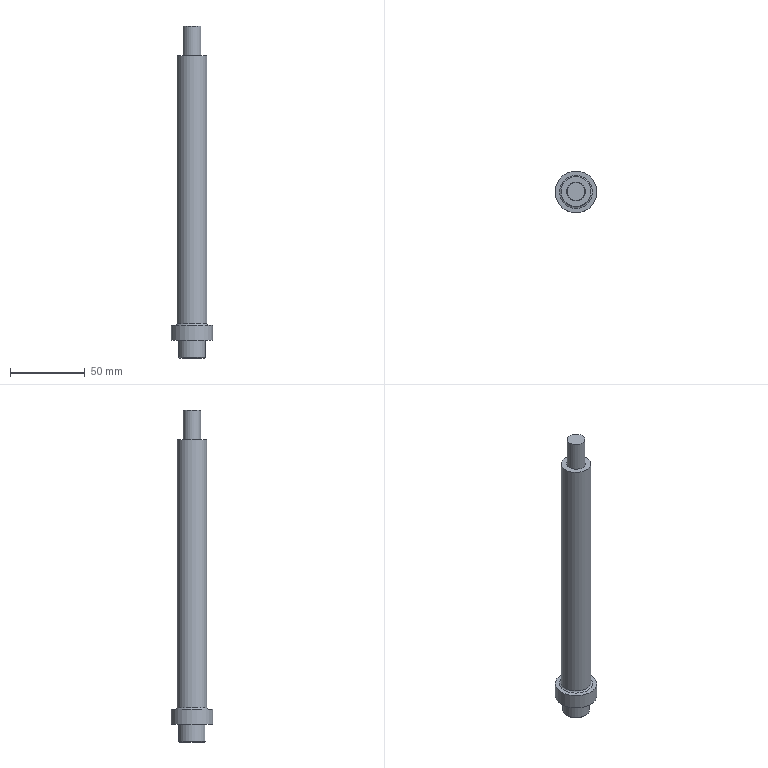Part | STEP file | 1_id3750_x_t | 1 solid | 29 faces | box 28 x 28 x 222 mm | volume 65272 mm3 | plane 18 | cylinder 6 | cone 4 | torus 1 | commonest cylinder face diameters 12.6 x2 12 x1 18 x1 20 x1 28 x1
STEP:
#1=CARTESIAN_POINT('',(2798.,0.00007613,-220.));
#2=VERTEX_POINT('',#1);
#3=CARTESIAN_POINT('',(2787.,0.00007613,-220.));
#4=DIRECTION('',(0.,0.,1.));
#5=DIRECTION('',(1.,0.,0.));
#6=AXIS2_PLACEMENT_3D('',#3,#4,#5);
#7=CIRCLE('',#6,11.);
#8=EDGE_CURVE('',#2,#2,#7,.T.);
#9=ORIENTED_EDGE('',*,*,#8,.T.);
#10=EDGE_LOOP('',(#9));
#11=FACE_BOUND('',#10,.T.);
#12=CARTESIAN_POINT('',(2797.,0.00007613,-219.));
#13=VERTEX_POINT('',#12);
#14=CARTESIAN_POINT('',(2787.,0.00007613,-219.));
#15=DIRECTION('',(0.,0.,-1.));
#16=DIRECTION('',(1.,0.,0.));
#17=AXIS2_PLACEMENT_3D('',#14,#15,#16);
#18=CIRCLE('',#17,10.);
#19=EDGE_CURVE('',#13,#13,#18,.T.);
#20=ORIENTED_EDGE('',*,*,#19,.T.);
#21=EDGE_LOOP('',(#20));
#22=FACE_BOUND('',#21,.T.);
#23=CARTESIAN_POINT('',(2787.,0.00007613,-219.));
#24=DIRECTION('',(0.,0.,-1.));
#25=DIRECTION('',(-1.,0.,0.));
#26=AXIS2_PLACEMENT_3D('',#23,#24,#25);
#27=TOROIDAL_SURFACE('',#26,11.,1.);
#28=ADVANCED_FACE('',(#11,#22),#27,.F.);
#29=CARTESIAN_POINT('',(2773.,0.00007613,-230.));
#30=VERTEX_POINT('',#29);
#31=CARTESIAN_POINT('',(2787.,0.00007613,-230.));
#32=DIRECTION('',(0.,0.,-1.));
#33=DIRECTION('',(-1.,0.,0.));
#34=AXIS2_PLACEMENT_3D('',#31,#32,#33);
#35=CIRCLE('',#34,14.);
#36=EDGE_CURVE('',#30,#30,#35,.T.);
#37=ORIENTED_EDGE('',*,*,#36,.F.);
#38=EDGE_LOOP('',(#37));
#39=FACE_BOUND('',#38,.T.);
#40=CARTESIAN_POINT('',(2773.,0.00007613,-220.));
#41=VERTEX_POINT('',#40);
#42=CARTESIAN_POINT('',(2787.,0.00007613,-220.));
#43=DIRECTION('',(0.,0.,1.));
#44=DIRECTION('',(-1.,0.,0.));
#45=AXIS2_PLACEMENT_3D('',#42,#43,#44);
#46=CIRCLE('',#45,14.);
#47=EDGE_CURVE('',#41,#41,#46,.T.);
#48=ORIENTED_EDGE('',*,*,#47,.F.);
#49=EDGE_LOOP('',(#48));
#50=FACE_BOUND('',#49,.T.);
#51=CARTESIAN_POINT('',(2787.,0.00007613,-225.));
#52=DIRECTION('',(0.,0.,1.));
#53=DIRECTION('',(1.,0.,0.));
#54=AXIS2_PLACEMENT_3D('',#51,#52,#53);
#55=CYLINDRICAL_SURFACE('',#54,14.);
#56=ADVANCED_FACE('',(#39,#50),#55,.T.);
#57=CARTESIAN_POINT('',(2780.7,0.00007613,-40.));
#58=VERTEX_POINT('',#57);
#59=CARTESIAN_POINT('',(2780.7,0.00007613,-230.));
#60=VERTEX_POINT('',#59);
#61=CARTESIAN_POINT('',(2780.7,0.00007613,-95.));
#62=DIRECTION('',(0.,0.,-1.));
#63=VECTOR('',#62,1.);
#64=LINE('',#61,#63);
#65=EDGE_CURVE('',#58,#60,#64,.T.);
#66=ORIENTED_EDGE('',*,*,#65,.F.);
#67=CARTESIAN_POINT('',(2793.3,0.00007613,-40.));
#68=VERTEX_POINT('',#67);
#69=CARTESIAN_POINT('',(2787.,0.00007613,-40.));
#70=DIRECTION('',(0.,0.,-1.));
#71=DIRECTION('',(-1.,0.,0.));
#72=AXIS2_PLACEMENT_3D('',#69,#70,#71);
#73=CIRCLE('',#72,6.3);
#74=EDGE_CURVE('',#68,#58,#73,.T.);
#75=ORIENTED_EDGE('',*,*,#74,.F.);
#76=CARTESIAN_POINT('',(2793.3,0.00007613,-230.));
#77=VERTEX_POINT('',#76);
#78=CARTESIAN_POINT('',(2793.3,0.00007613,-95.));
#79=DIRECTION('',(0.,0.,1.));
#80=VECTOR('',#79,1.);
#81=LINE('',#78,#80);
#82=EDGE_CURVE('',#77,#68,#81,.T.);
#83=ORIENTED_EDGE('',*,*,#82,.F.);
#84=CARTESIAN_POINT('',(2787.,0.00007613,-230.));
#85=DIRECTION('',(0.,0.,1.));
#86=DIRECTION('',(-1.,0.,0.));
#87=AXIS2_PLACEMENT_3D('',#84,#85,#86);
#88=CIRCLE('',#87,6.3);
#89=EDGE_CURVE('',#60,#77,#88,.T.);
#90=ORIENTED_EDGE('',*,*,#89,.F.);
#91=EDGE_LOOP('',(#66,#75,#83,#90));
#92=FACE_OUTER_BOUND('',#91,.T.);
#93=CARTESIAN_POINT('',(2787.,0.00007613,-95.));
#94=DIRECTION('',(0.,0.,1.));
#95=DIRECTION('',(1.,0.,0.));
#96=AXIS2_PLACEMENT_3D('',#93,#94,#95);
#97=CYLINDRICAL_SURFACE('',#96,6.3);
#98=ADVANCED_FACE('',(#92),#97,.F.);
#99=ORIENTED_EDGE('',*,*,#19,.F.);
#100=EDGE_LOOP('',(#99));
#101=FACE_BOUND('',#100,.T.);
#102=CARTESIAN_POINT('',(2777.,0.00007613,-40.));
#103=VERTEX_POINT('',#102);
#104=CARTESIAN_POINT('',(2787.,0.00007613,-40.));
#105=DIRECTION('',(0.,0.,1.));
#106=DIRECTION('',(-1.,0.,0.));
#107=AXIS2_PLACEMENT_3D('',#104,#105,#106);
#108=CIRCLE('',#107,10.);
#109=EDGE_CURVE('',#103,#103,#108,.T.);
#110=ORIENTED_EDGE('',*,*,#109,.F.);
#111=EDGE_LOOP('',(#110));
#112=FACE_BOUND('',#111,.T.);
#113=CARTESIAN_POINT('',(2787.,0.00007613,-90.));
#114=DIRECTION('',(0.,0.,1.));
#115=DIRECTION('',(1.,0.,0.));
#116=AXIS2_PLACEMENT_3D('',#113,#114,#115);
#117=CYLINDRICAL_SURFACE('',#116,10.);
#118=ADVANCED_FACE('',(#101,#112),#117,.T.);
#119=CARTESIAN_POINT('',(2781.,0.00007613,-230.));
#120=VERTEX_POINT('',#119);
#121=CARTESIAN_POINT('',(2787.,0.00007613,-230.));
#122=DIRECTION('',(0.,0.,-1.));
#123=DIRECTION('',(-1.,0.,0.));
#124=AXIS2_PLACEMENT_3D('',#121,#122,#123);
#125=CIRCLE('',#124,6.);
#126=EDGE_CURVE('',#120,#120,#125,.T.);
#127=ORIENTED_EDGE('',*,*,#126,.F.);
#128=EDGE_LOOP('',(#127));
#129=FACE_BOUND('',#128,.T.);
#130=CARTESIAN_POINT('',(2781.,0.00007613,-20.));
#131=VERTEX_POINT('',#130);
#132=CARTESIAN_POINT('',(2787.,0.00007613,-20.));
#133=DIRECTION('',(0.,0.,1.));
#134=DIRECTION('',(-1.,0.,0.));
#135=AXIS2_PLACEMENT_3D('',#132,#133,#134);
#136=CIRCLE('',#135,6.);
#137=EDGE_CURVE('',#131,#131,#136,.T.);
#138=ORIENTED_EDGE('',*,*,#137,.F.);
#139=EDGE_LOOP('',(#138));
#140=FACE_BOUND('',#139,.T.);
#141=CARTESIAN_POINT('',(2787.,0.00007613,-85.));
#142=DIRECTION('',(0.,0.,1.));
#143=DIRECTION('',(1.,0.,0.));
#144=AXIS2_PLACEMENT_3D('',#141,#142,#143);
#145=CYLINDRICAL_SURFACE('',#144,6.);
#146=ADVANCED_FACE('',(#129,#140),#145,.T.);
#147=CARTESIAN_POINT('',(2792.774,0.00007613,-236.));
#148=VERTEX_POINT('',#147);
#149=CARTESIAN_POINT('',(2787.,0.00007613,-235.));
#150=VERTEX_POINT('',#149);
#151=CARTESIAN_POINT('',(2789.887,0.00007613,-235.5));
#152=DIRECTION('',(-0.9853,0.,0.1707));
#153=VECTOR('',#152,1.);
#154=LINE('',#151,#153);
#155=EDGE_CURVE('',#148,#150,#154,.T.);
#156=ORIENTED_EDGE('',*,*,#155,.T.);
#157=CARTESIAN_POINT('',(2781.226,0.00007613,-236.));
#158=VERTEX_POINT('',#157);
#159=CARTESIAN_POINT('',(2784.113,0.00007613,-235.5));
#160=DIRECTION('',(-0.9853,0.,-0.1707));
#161=VECTOR('',#160,1.);
#162=LINE('',#159,#161);
#163=EDGE_CURVE('',#150,#158,#162,.T.);
#164=ORIENTED_EDGE('',*,*,#163,.T.);
#165=CARTESIAN_POINT('',(2782.,2.887,-236.));
#166=VERTEX_POINT('',#165);
#167=CARTESIAN_POINT('',(2787.,0.00007613,-236.));
#168=DIRECTION('',(0.,0.,-1.));
#169=DIRECTION('',(-1.,0.,0.));
#170=AXIS2_PLACEMENT_3D('',#167,#168,#169);
#171=CIRCLE('',#170,5.774);
#172=EDGE_CURVE('',#158,#166,#171,.T.);
#173=ORIENTED_EDGE('',*,*,#172,.T.);
#174=CARTESIAN_POINT('',(2787.,5.774,-236.));
#175=VERTEX_POINT('',#174);
#176=CARTESIAN_POINT('',(2787.,0.00007613,-236.));
#177=DIRECTION('',(0.,0.,-1.));
#178=DIRECTION('',(-1.,0.,0.));
#179=AXIS2_PLACEMENT_3D('',#176,#177,#178);
#180=CIRCLE('',#179,5.774);
#181=EDGE_CURVE('',#166,#175,#180,.T.);
#182=ORIENTED_EDGE('',*,*,#181,.T.);
#183=CARTESIAN_POINT('',(2792.,2.887,-236.));
#184=VERTEX_POINT('',#183);
#185=CARTESIAN_POINT('',(2787.,0.00007613,-236.));
#186=DIRECTION('',(0.,0.,-1.));
#187=DIRECTION('',(-1.,0.,0.));
#188=AXIS2_PLACEMENT_3D('',#185,#186,#187);
#189=CIRCLE('',#188,5.774);
#190=EDGE_CURVE('',#175,#184,#189,.T.);
#191=ORIENTED_EDGE('',*,*,#190,.T.);
#192=CARTESIAN_POINT('',(2787.,0.00007613,-236.));
#193=DIRECTION('',(0.,0.,-1.));
#194=DIRECTION('',(-1.,0.,0.));
#195=AXIS2_PLACEMENT_3D('',#192,#193,#194);
#196=CIRCLE('',#195,5.774);
#197=EDGE_CURVE('',#184,#148,#196,.T.);
#198=ORIENTED_EDGE('',*,*,#197,.T.);
#199=EDGE_LOOP('',(#156,#164,#173,#182,#191,#198));
#200=FACE_OUTER_BOUND('',#199,.T.);
#201=CARTESIAN_POINT('',(2787.,0.00007613,-235.5));
#202=DIRECTION('',(0.,0.,-1.));
#203=DIRECTION('',(1.,0.,0.));
#204=AXIS2_PLACEMENT_3D('',#201,#202,#203);
#205=CONICAL_SURFACE('',#204,2.887,80.174);
#206=ADVANCED_FACE('',(#200),#205,.F.);
#207=CARTESIAN_POINT('',(2778.,0.00007613,-241.5));
#208=VERTEX_POINT('',#207);
#209=CARTESIAN_POINT('',(2796.,0.00007613,-241.5));
#210=VERTEX_POINT('',#209);
#211=CARTESIAN_POINT('',(2787.,0.00007613,-241.5));
#212=DIRECTION('',(0.,0.,-1.));
#213=DIRECTION('',(1.,0.,0.));
#214=AXIS2_PLACEMENT_3D('',#211,#212,#213);
#215=CIRCLE('',#214,9.);
#216=EDGE_CURVE('',#208,#210,#215,.T.);
#217=ORIENTED_EDGE('',*,*,#216,.F.);
#218=CARTESIAN_POINT('',(2787.,0.00007613,-241.5));
#219=DIRECTION('',(0.,0.,-1.));
#220=DIRECTION('',(1.,0.,0.));
#221=AXIS2_PLACEMENT_3D('',#218,#219,#220);
#222=CIRCLE('',#221,9.);
#223=EDGE_CURVE('',#210,#208,#222,.T.);
#224=ORIENTED_EDGE('',*,*,#223,.F.);
#225=EDGE_LOOP('',(#217,#224));
#226=FACE_BOUND('',#225,.T.);
#227=CARTESIAN_POINT('',(2778.,0.00007613,-230.));
#228=VERTEX_POINT('',#227);
#229=CARTESIAN_POINT('',(2787.,0.00007613,-230.));
#230=DIRECTION('',(0.,0.,1.));
#231=DIRECTION('',(-1.,0.,0.));
#232=AXIS2_PLACEMENT_3D('',#229,#230,#231);
#233=CIRCLE('',#232,9.);
#234=EDGE_CURVE('',#228,#228,#233,.T.);
#235=ORIENTED_EDGE('',*,*,#234,.F.);
#236=EDGE_LOOP('',(#235));
#237=FACE_BOUND('',#236,.T.);
#238=CARTESIAN_POINT('',(2787.,0.00007613,-236.));
#239=DIRECTION('',(0.,0.,1.));
#240=DIRECTION('',(1.,0.,0.));
#241=AXIS2_PLACEMENT_3D('',#238,#239,#240);
#242=CYLINDRICAL_SURFACE('',#241,9.);
#243=ADVANCED_FACE('',(#226,#237),#242,.T.);
#244=CARTESIAN_POINT('',(2795.5,0.00007613,-242.));
#245=VERTEX_POINT('',#244);
#246=CARTESIAN_POINT('',(2795.5,0.00007613,-242.));
#247=DIRECTION('',(-0.7071,0.,-0.7071));
#248=VECTOR('',#247,1.);
#249=LINE('',#246,#248);
#250=EDGE_CURVE('',#210,#245,#249,.T.);
#251=ORIENTED_EDGE('',*,*,#250,.F.);
#252=ORIENTED_EDGE('',*,*,#223,.T.);
#253=CARTESIAN_POINT('',(2778.5,0.00007613,-242.));
#254=VERTEX_POINT('',#253);
#255=CARTESIAN_POINT('',(2778.5,0.00007613,-242.));
#256=DIRECTION('',(-0.7071,0.,0.7071));
#257=VECTOR('',#256,1.);
#258=LINE('',#255,#257);
#259=EDGE_CURVE('',#254,#208,#258,.T.);
#260=ORIENTED_EDGE('',*,*,#259,.F.);
#261=CARTESIAN_POINT('',(2787.,0.00007613,-242.));
#262=DIRECTION('',(0.,0.,1.));
#263=DIRECTION('',(1.,0.,0.));
#264=AXIS2_PLACEMENT_3D('',#261,#262,#263);
#265=CIRCLE('',#264,8.5);
#266=EDGE_CURVE('',#254,#245,#265,.T.);
#267=ORIENTED_EDGE('',*,*,#266,.T.);
#268=EDGE_LOOP('',(#251,#252,#260,#267));
#269=FACE_OUTER_BOUND('',#268,.T.);
#270=CARTESIAN_POINT('',(2787.,0.00007613,-242.));
#271=DIRECTION('',(0.,0.,1.));
#272=DIRECTION('',(-1.,0.,0.));
#273=AXIS2_PLACEMENT_3D('',#270,#271,#272);
#274=CONICAL_SURFACE('',#273,8.5,45.);
#275=ADVANCED_FACE('',(#269),#274,.T.);
#276=ORIENTED_EDGE('',*,*,#126,.T.);
#277=EDGE_LOOP('',(#276));
#278=FACE_BOUND('',#277,.T.);
#279=ORIENTED_EDGE('',*,*,#89,.T.);
#280=CARTESIAN_POINT('',(2787.,0.00007613,-230.));
#281=DIRECTION('',(0.,0.,1.));
#282=DIRECTION('',(-1.,0.,0.));
#283=AXIS2_PLACEMENT_3D('',#280,#281,#282);
#284=CIRCLE('',#283,6.3);
#285=EDGE_CURVE('',#77,#60,#284,.T.);
#286=ORIENTED_EDGE('',*,*,#285,.T.);
#287=EDGE_LOOP('',(#279,#286));
#288=FACE_BOUND('',#287,.T.);
#289=CARTESIAN_POINT('',(2787.,0.00007613,-230.));
#290=DIRECTION('',(0.,0.,1.));
#291=DIRECTION('',(1.,0.,0.));
#292=AXIS2_PLACEMENT_3D('',#289,#290,#291);
#293=PLANE('',#292);
#294=ADVANCED_FACE('',(#278,#288),#293,.T.);
#295=ORIENTED_EDGE('',*,*,#250,.T.);
#296=CARTESIAN_POINT('',(2787.,0.00007613,-242.));
#297=DIRECTION('',(0.,0.,1.));
#298=DIRECTION('',(1.,0.,0.));
#299=AXIS2_PLACEMENT_3D('',#296,#297,#298);
#300=CIRCLE('',#299,8.5);
#301=EDGE_CURVE('',#245,#254,#300,.T.);
#302=ORIENTED_EDGE('',*,*,#301,.T.);
#303=ORIENTED_EDGE('',*,*,#259,.T.);
#304=ORIENTED_EDGE('',*,*,#216,.T.);
#305=EDGE_LOOP('',(#295,#302,#303,#304));
#306=FACE_OUTER_BOUND('',#305,.T.);
#307=CARTESIAN_POINT('',(2787.,0.00007613,-242.));
#308=DIRECTION('',(0.,0.,1.));
#309=DIRECTION('',(-1.,0.,0.));
#310=AXIS2_PLACEMENT_3D('',#307,#308,#309);
#311=CONICAL_SURFACE('',#310,8.5,45.);
#312=ADVANCED_FACE('',(#306),#311,.T.);
#313=CARTESIAN_POINT('',(2787.,5.774,-242.));
#314=VERTEX_POINT('',#313);
#315=CARTESIAN_POINT('',(2782.,2.887,-242.));
#316=VERTEX_POINT('',#315);
#317=CARTESIAN_POINT('',(2784.5,4.33,-242.));
#318=DIRECTION('',(-0.866,-0.5,0.));
#319=VECTOR('',#318,1.);
#320=LINE('',#317,#319);
#321=EDGE_CURVE('',#314,#316,#320,.T.);
#322=ORIENTED_EDGE('',*,*,#321,.T.);
#323=CARTESIAN_POINT('',(2782.,-2.887,-242.));
#324=VERTEX_POINT('',#323);
#325=CARTESIAN_POINT('',(2782.,0.00007613,-242.));
#326=DIRECTION('',(0.,-1.,0.));
#327=VECTOR('',#326,1.);
#328=LINE('',#325,#327);
#329=EDGE_CURVE('',#316,#324,#328,.T.);
#330=ORIENTED_EDGE('',*,*,#329,.T.);
#331=CARTESIAN_POINT('',(2787.,-5.773,-242.));
#332=VERTEX_POINT('',#331);
#333=CARTESIAN_POINT('',(2784.5,-4.33,-242.));
#334=DIRECTION('',(0.866,-0.5,0.));
#335=VECTOR('',#334,1.);
#336=LINE('',#333,#335);
#337=EDGE_CURVE('',#324,#332,#336,.T.);
#338=ORIENTED_EDGE('',*,*,#337,.T.);
#339=CARTESIAN_POINT('',(2792.,-2.887,-242.));
#340=VERTEX_POINT('',#339);
#341=CARTESIAN_POINT('',(2789.5,-4.33,-242.));
#342=DIRECTION('',(0.866,0.5,0.));
#343=VECTOR('',#342,1.);
#344=LINE('',#341,#343);
#345=EDGE_CURVE('',#332,#340,#344,.T.);
#346=ORIENTED_EDGE('',*,*,#345,.T.);
#347=CARTESIAN_POINT('',(2792.,2.887,-242.));
#348=VERTEX_POINT('',#347);
#349=CARTESIAN_POINT('',(2792.,0.00007613,-242.));
#350=DIRECTION('',(0.,1.,0.));
#351=VECTOR('',#350,1.);
#352=LINE('',#349,#351);
#353=EDGE_CURVE('',#340,#348,#352,.T.);
#354=ORIENTED_EDGE('',*,*,#353,.T.);
#355=CARTESIAN_POINT('',(2789.5,4.33,-242.));
#356=DIRECTION('',(-0.866,0.5,0.));
#357=VECTOR('',#356,1.);
#358=LINE('',#355,#357);
#359=EDGE_CURVE('',#348,#314,#358,.T.);
#360=ORIENTED_EDGE('',*,*,#359,.T.);
#361=EDGE_LOOP('',(#322,#330,#338,#346,#354,#360));
#362=FACE_BOUND('',#361,.T.);
#363=ORIENTED_EDGE('',*,*,#266,.F.);
#364=ORIENTED_EDGE('',*,*,#301,.F.);
#365=EDGE_LOOP('',(#363,#364));
#366=FACE_BOUND('',#365,.T.);
#367=CARTESIAN_POINT('',(2787.,0.00007613,-242.));
#368=DIRECTION('',(0.,0.,-1.));
#369=DIRECTION('',(-1.,0.,0.));
#370=AXIS2_PLACEMENT_3D('',#367,#368,#369);
#371=PLANE('',#370);
#372=ADVANCED_FACE('',(#362,#366),#371,.T.);
#373=CARTESIAN_POINT('',(2784.5,4.33,-236.));
#374=DIRECTION('',(-0.866,-0.5,0.));
#375=VECTOR('',#374,1.);
#376=LINE('',#373,#375);
#377=EDGE_CURVE('',#175,#166,#376,.T.);
#378=ORIENTED_EDGE('',*,*,#377,.F.);
#379=ORIENTED_EDGE('',*,*,#181,.F.);
#380=EDGE_LOOP('',(#378,#379));
#381=FACE_OUTER_BOUND('',#380,.T.);
#382=CARTESIAN_POINT('',(2787.,0.00007613,-236.));
#383=DIRECTION('',(0.,0.,-1.));
#384=DIRECTION('',(-1.,0.,0.));
#385=AXIS2_PLACEMENT_3D('',#382,#383,#384);
#386=PLANE('',#385);
#387=ADVANCED_FACE('',(#381),#386,.F.);
#388=CARTESIAN_POINT('',(2782.,-2.887,-236.));
#389=VERTEX_POINT('',#388);
#390=CARTESIAN_POINT('',(2782.,0.00007613,-236.));
#391=DIRECTION('',(0.,-1.,0.));
#392=VECTOR('',#391,1.);
#393=LINE('',#390,#392);
#394=EDGE_CURVE('',#166,#389,#393,.T.);
#395=ORIENTED_EDGE('',*,*,#394,.F.);
#396=ORIENTED_EDGE('',*,*,#172,.F.);
#397=CARTESIAN_POINT('',(2787.,0.00007613,-236.));
#398=DIRECTION('',(0.,0.,-1.));
#399=DIRECTION('',(-1.,0.,0.));
#400=AXIS2_PLACEMENT_3D('',#397,#398,#399);
#401=CIRCLE('',#400,5.774);
#402=EDGE_CURVE('',#389,#158,#401,.T.);
#403=ORIENTED_EDGE('',*,*,#402,.F.);
#404=EDGE_LOOP('',(#395,#396,#403));
#405=FACE_OUTER_BOUND('',#404,.T.);
#406=CARTESIAN_POINT('',(2787.,0.00007613,-236.));
#407=DIRECTION('',(0.,0.,-1.));
#408=DIRECTION('',(-1.,0.,0.));
#409=AXIS2_PLACEMENT_3D('',#406,#407,#408);
#410=PLANE('',#409);
#411=ADVANCED_FACE('',(#405),#410,.F.);
#412=CARTESIAN_POINT('',(2787.,-5.773,-236.));
#413=VERTEX_POINT('',#412);
#414=CARTESIAN_POINT('',(2784.5,-4.33,-236.));
#415=DIRECTION('',(0.866,-0.5,0.));
#416=VECTOR('',#415,1.);
#417=LINE('',#414,#416);
#418=EDGE_CURVE('',#389,#413,#417,.T.);
#419=ORIENTED_EDGE('',*,*,#418,.F.);
#420=CARTESIAN_POINT('',(2787.,0.00007613,-236.));
#421=DIRECTION('',(0.,0.,-1.));
#422=DIRECTION('',(-1.,0.,0.));
#423=AXIS2_PLACEMENT_3D('',#420,#421,#422);
#424=CIRCLE('',#423,5.774);
#425=EDGE_CURVE('',#413,#389,#424,.T.);
#426=ORIENTED_EDGE('',*,*,#425,.F.);
#427=EDGE_LOOP('',(#419,#426));
#428=FACE_OUTER_BOUND('',#427,.T.);
#429=CARTESIAN_POINT('',(2787.,0.00007613,-236.));
#430=DIRECTION('',(0.,0.,-1.));
#431=DIRECTION('',(-1.,0.,0.));
#432=AXIS2_PLACEMENT_3D('',#429,#430,#431);
#433=PLANE('',#432);
#434=ADVANCED_FACE('',(#428),#433,.F.);
#435=CARTESIAN_POINT('',(2792.,-2.887,-236.));
#436=VERTEX_POINT('',#435);
#437=CARTESIAN_POINT('',(2789.5,-4.33,-236.));
#438=DIRECTION('',(0.866,0.5,0.));
#439=VECTOR('',#438,1.);
#440=LINE('',#437,#439);
#441=EDGE_CURVE('',#413,#436,#440,.T.);
#442=ORIENTED_EDGE('',*,*,#441,.F.);
#443=CARTESIAN_POINT('',(2787.,0.00007613,-236.));
#444=DIRECTION('',(0.,0.,-1.));
#445=DIRECTION('',(-1.,0.,0.));
#446=AXIS2_PLACEMENT_3D('',#443,#444,#445);
#447=CIRCLE('',#446,5.774);
#448=EDGE_CURVE('',#436,#413,#447,.T.);
#449=ORIENTED_EDGE('',*,*,#448,.F.);
#450=EDGE_LOOP('',(#442,#449));
#451=FACE_OUTER_BOUND('',#450,.T.);
#452=CARTESIAN_POINT('',(2787.,0.00007613,-236.));
#453=DIRECTION('',(0.,0.,-1.));
#454=DIRECTION('',(-1.,0.,0.));
#455=AXIS2_PLACEMENT_3D('',#452,#453,#454);
#456=PLANE('',#455);
#457=ADVANCED_FACE('',(#451),#456,.F.);
#458=CARTESIAN_POINT('',(2792.,0.00007613,-236.));
#459=DIRECTION('',(0.,1.,0.));
#460=VECTOR('',#459,1.);
#461=LINE('',#458,#460);
#462=EDGE_CURVE('',#436,#184,#461,.T.);
#463=ORIENTED_EDGE('',*,*,#462,.F.);
#464=CARTESIAN_POINT('',(2787.,0.00007613,-236.));
#465=DIRECTION('',(0.,0.,-1.));
#466=DIRECTION('',(-1.,0.,0.));
#467=AXIS2_PLACEMENT_3D('',#464,#465,#466);
#468=CIRCLE('',#467,5.774);
#469=EDGE_CURVE('',#148,#436,#468,.T.);
#470=ORIENTED_EDGE('',*,*,#469,.F.);
#471=ORIENTED_EDGE('',*,*,#197,.F.);
#472=EDGE_LOOP('',(#463,#470,#471));
#473=FACE_OUTER_BOUND('',#472,.T.);
#474=CARTESIAN_POINT('',(2787.,0.00007613,-236.));
#475=DIRECTION('',(0.,0.,-1.));
#476=DIRECTION('',(-1.,0.,0.));
#477=AXIS2_PLACEMENT_3D('',#474,#475,#476);
#478=PLANE('',#477);
#479=ADVANCED_FACE('',(#473),#478,.F.);
#480=CARTESIAN_POINT('',(2789.5,4.33,-236.));
#481=DIRECTION('',(-0.866,0.5,0.));
#482=VECTOR('',#481,1.);
#483=LINE('',#480,#482);
#484=EDGE_CURVE('',#184,#175,#483,.T.);
#485=ORIENTED_EDGE('',*,*,#484,.F.);
#486=ORIENTED_EDGE('',*,*,#190,.F.);
#487=EDGE_LOOP('',(#485,#486));
#488=FACE_OUTER_BOUND('',#487,.T.);
#489=CARTESIAN_POINT('',(2787.,0.00007613,-236.));
#490=DIRECTION('',(0.,0.,-1.));
#491=DIRECTION('',(-1.,0.,0.));
#492=AXIS2_PLACEMENT_3D('',#489,#490,#491);
#493=PLANE('',#492);
#494=ADVANCED_FACE('',(#488),#493,.F.);
#495=ORIENTED_EDGE('',*,*,#155,.F.);
#496=ORIENTED_EDGE('',*,*,#469,.T.);
#497=ORIENTED_EDGE('',*,*,#448,.T.);
#498=ORIENTED_EDGE('',*,*,#425,.T.);
#499=ORIENTED_EDGE('',*,*,#402,.T.);
#500=ORIENTED_EDGE('',*,*,#163,.F.);
#501=EDGE_LOOP('',(#495,#496,#497,#498,#499,#500));
#502=FACE_OUTER_BOUND('',#501,.T.);
#503=CARTESIAN_POINT('',(2787.,0.00007613,-235.5));
#504=DIRECTION('',(0.,0.,-1.));
#505=DIRECTION('',(1.,0.,0.));
#506=AXIS2_PLACEMENT_3D('',#503,#504,#505);
#507=CONICAL_SURFACE('',#506,2.887,80.174);
#508=ADVANCED_FACE('',(#502),#507,.F.);
#509=CARTESIAN_POINT('',(2787.,5.774,-239.));
#510=DIRECTION('',(0.,0.,-1.));
#511=VECTOR('',#510,1.);
#512=LINE('',#509,#511);
#513=EDGE_CURVE('',#175,#314,#512,.T.);
#514=ORIENTED_EDGE('',*,*,#513,.F.);
#515=ORIENTED_EDGE('',*,*,#377,.T.);
#516=CARTESIAN_POINT('',(2782.,2.887,-239.));
#517=DIRECTION('',(0.,0.,-1.));
#518=VECTOR('',#517,1.);
#519=LINE('',#516,#518);
#520=EDGE_CURVE('',#166,#316,#519,.T.);
#521=ORIENTED_EDGE('',*,*,#520,.T.);
#522=ORIENTED_EDGE('',*,*,#321,.F.);
#523=EDGE_LOOP('',(#514,#515,#521,#522));
#524=FACE_OUTER_BOUND('',#523,.T.);
#525=CARTESIAN_POINT('',(2784.5,4.33,-239.));
#526=DIRECTION('',(0.5,-0.866,0.));
#527=DIRECTION('',(0.,0.,-1.));
#528=AXIS2_PLACEMENT_3D('',#525,#526,#527);
#529=PLANE('',#528);
#530=ADVANCED_FACE('',(#524),#529,.T.);
#531=CARTESIAN_POINT('',(2792.,2.887,-239.));
#532=DIRECTION('',(0.,0.,-1.));
#533=VECTOR('',#532,1.);
#534=LINE('',#531,#533);
#535=EDGE_CURVE('',#184,#348,#534,.T.);
#536=ORIENTED_EDGE('',*,*,#535,.F.);
#537=ORIENTED_EDGE('',*,*,#484,.T.);
#538=ORIENTED_EDGE('',*,*,#513,.T.);
#539=ORIENTED_EDGE('',*,*,#359,.F.);
#540=EDGE_LOOP('',(#536,#537,#538,#539));
#541=FACE_OUTER_BOUND('',#540,.T.);
#542=CARTESIAN_POINT('',(2789.5,4.33,-239.));
#543=DIRECTION('',(-0.5,-0.866,0.));
#544=DIRECTION('',(0.,0.,1.));
#545=AXIS2_PLACEMENT_3D('',#542,#543,#544);
#546=PLANE('',#545);
#547=ADVANCED_FACE('',(#541),#546,.T.);
#548=CARTESIAN_POINT('',(2792.,-2.887,-239.));
#549=DIRECTION('',(0.,0.,-1.));
#550=VECTOR('',#549,1.);
#551=LINE('',#548,#550);
#552=EDGE_CURVE('',#436,#340,#551,.T.);
#553=ORIENTED_EDGE('',*,*,#552,.F.);
#554=ORIENTED_EDGE('',*,*,#462,.T.);
#555=ORIENTED_EDGE('',*,*,#535,.T.);
#556=ORIENTED_EDGE('',*,*,#353,.F.);
#557=EDGE_LOOP('',(#553,#554,#555,#556));
#558=FACE_OUTER_BOUND('',#557,.T.);
#559=CARTESIAN_POINT('',(2792.,0.00007613,-239.));
#560=DIRECTION('',(-1.,0.,0.));
#561=DIRECTION('',(0.,0.,1.));
#562=AXIS2_PLACEMENT_3D('',#559,#560,#561);
#563=PLANE('',#562);
#564=ADVANCED_FACE('',(#558),#563,.T.);
#565=CARTESIAN_POINT('',(2787.,-5.773,-239.));
#566=DIRECTION('',(0.,0.,-1.));
#567=VECTOR('',#566,1.);
#568=LINE('',#565,#567);
#569=EDGE_CURVE('',#413,#332,#568,.T.);
#570=ORIENTED_EDGE('',*,*,#569,.F.);
#571=ORIENTED_EDGE('',*,*,#441,.T.);
#572=ORIENTED_EDGE('',*,*,#552,.T.);
#573=ORIENTED_EDGE('',*,*,#345,.F.);
#574=EDGE_LOOP('',(#570,#571,#572,#573));
#575=FACE_OUTER_BOUND('',#574,.T.);
#576=CARTESIAN_POINT('',(2789.5,-4.33,-239.));
#577=DIRECTION('',(-0.5,0.866,0.));
#578=DIRECTION('',(0.,0.,1.));
#579=AXIS2_PLACEMENT_3D('',#576,#577,#578);
#580=PLANE('',#579);
#581=ADVANCED_FACE('',(#575),#580,.T.);
#582=CARTESIAN_POINT('',(2782.,-2.887,-239.));
#583=DIRECTION('',(0.,0.,-1.));
#584=VECTOR('',#583,1.);
#585=LINE('',#582,#584);
#586=EDGE_CURVE('',#389,#324,#585,.T.);
#587=ORIENTED_EDGE('',*,*,#586,.F.);
#588=ORIENTED_EDGE('',*,*,#418,.T.);
#589=ORIENTED_EDGE('',*,*,#569,.T.);
#590=ORIENTED_EDGE('',*,*,#337,.F.);
#591=EDGE_LOOP('',(#587,#588,#589,#590));
#592=FACE_OUTER_BOUND('',#591,.T.);
#593=CARTESIAN_POINT('',(2784.5,-4.33,-239.));
#594=DIRECTION('',(0.5,0.866,0.));
#595=DIRECTION('',(0.,0.,-1.));
#596=AXIS2_PLACEMENT_3D('',#593,#594,#595);
#597=PLANE('',#596);
#598=ADVANCED_FACE('',(#592),#597,.T.);
#599=ORIENTED_EDGE('',*,*,#520,.F.);
#600=ORIENTED_EDGE('',*,*,#394,.T.);
#601=ORIENTED_EDGE('',*,*,#586,.T.);
#602=ORIENTED_EDGE('',*,*,#329,.F.);
#603=EDGE_LOOP('',(#599,#600,#601,#602));
#604=FACE_OUTER_BOUND('',#603,.T.);
#605=CARTESIAN_POINT('',(2782.,0.00007613,-239.));
#606=DIRECTION('',(1.,0.,0.));
#607=DIRECTION('',(0.,0.,-1.));
#608=AXIS2_PLACEMENT_3D('',#605,#606,#607);
#609=PLANE('',#608);
#610=ADVANCED_FACE('',(#604),#609,.T.);
#611=ORIENTED_EDGE('',*,*,#137,.T.);
#612=EDGE_LOOP('',(#611));
#613=FACE_OUTER_BOUND('',#612,.T.);
#614=CARTESIAN_POINT('',(2787.,0.00007613,-20.));
#615=DIRECTION('',(0.,0.,1.));
#616=DIRECTION('',(1.,0.,0.));
#617=AXIS2_PLACEMENT_3D('',#614,#615,#616);
#618=PLANE('',#617);
#619=ADVANCED_FACE('',(#613),#618,.T.);
#620=ORIENTED_EDGE('',*,*,#47,.T.);
#621=EDGE_LOOP('',(#620));
#622=FACE_BOUND('',#621,.T.);
#623=ORIENTED_EDGE('',*,*,#8,.F.);
#624=EDGE_LOOP('',(#623));
#625=FACE_BOUND('',#624,.T.);
#626=CARTESIAN_POINT('',(2787.,0.00007613,-220.));
#627=DIRECTION('',(0.,0.,1.));
#628=DIRECTION('',(1.,0.,0.));
#629=AXIS2_PLACEMENT_3D('',#626,#627,#628);
#630=PLANE('',#629);
#631=ADVANCED_FACE('',(#622,#625),#630,.T.);
#632=ORIENTED_EDGE('',*,*,#65,.T.);
#633=ORIENTED_EDGE('',*,*,#285,.F.);
#634=ORIENTED_EDGE('',*,*,#82,.T.);
#635=CARTESIAN_POINT('',(2787.,0.00007613,-40.));
#636=DIRECTION('',(0.,0.,-1.));
#637=DIRECTION('',(-1.,0.,0.));
#638=AXIS2_PLACEMENT_3D('',#635,#636,#637);
#639=CIRCLE('',#638,6.3);
#640=EDGE_CURVE('',#58,#68,#639,.T.);
#641=ORIENTED_EDGE('',*,*,#640,.F.);
#642=EDGE_LOOP('',(#632,#633,#634,#641));
#643=FACE_OUTER_BOUND('',#642,.T.);
#644=CARTESIAN_POINT('',(2787.,0.00007613,-95.));
#645=DIRECTION('',(0.,0.,1.));
#646=DIRECTION('',(1.,0.,0.));
#647=AXIS2_PLACEMENT_3D('',#644,#645,#646);
#648=CYLINDRICAL_SURFACE('',#647,6.3);
#649=ADVANCED_FACE('',(#643),#648,.F.);
#650=ORIENTED_EDGE('',*,*,#640,.T.);
#651=ORIENTED_EDGE('',*,*,#74,.T.);
#652=EDGE_LOOP('',(#650,#651));
#653=FACE_BOUND('',#652,.T.);
#654=ORIENTED_EDGE('',*,*,#109,.T.);
#655=EDGE_LOOP('',(#654));
#656=FACE_BOUND('',#655,.T.);
#657=CARTESIAN_POINT('',(2787.,0.00007613,-40.));
#658=DIRECTION('',(0.,0.,1.));
#659=DIRECTION('',(1.,0.,0.));
#660=AXIS2_PLACEMENT_3D('',#657,#658,#659);
#661=PLANE('',#660);
#662=ADVANCED_FACE('',(#653,#656),#661,.T.);
#663=ORIENTED_EDGE('',*,*,#234,.T.);
#664=EDGE_LOOP('',(#663));
#665=FACE_BOUND('',#664,.T.);
#666=ORIENTED_EDGE('',*,*,#36,.T.);
#667=EDGE_LOOP('',(#666));
#668=FACE_BOUND('',#667,.T.);
#669=CARTESIAN_POINT('',(2787.,0.00007613,-230.));
#670=DIRECTION('',(0.,0.,-1.));
#671=DIRECTION('',(-1.,0.,0.));
#672=AXIS2_PLACEMENT_3D('',#669,#670,#671);
#673=PLANE('',#672);
#674=ADVANCED_FACE('',(#665,#668),#673,.T.);
#675=CLOSED_SHELL('',(#28,#56,#98,#118,#146,#206,#243,#275,#294,#312,#372,#387,#411,#434,#457,#479,#494,#508,#530,#547,#564,#581,#598,#610,#619,#631,#649,#662,#674));
#676=MANIFOLD_SOLID_BREP('',#675);
#677=(LENGTH_UNIT()NAMED_UNIT(*)SI_UNIT(.MILLI.,.METRE.));
#678=UNCERTAINTY_MEASURE_WITH_UNIT(LENGTH_MEASURE(0.00002),#677,'','');
#679=(NAMED_UNIT(*)PLANE_ANGLE_UNIT()SI_UNIT($,.RADIAN.));
#680=PLANE_ANGLE_MEASURE_WITH_UNIT(PLANE_ANGLE_MEASURE(0.01745),#679);
#681=DIMENSIONAL_EXPONENTS(0.,0.,0.,0.,0.,0.,0.);
#682=(CONVERSION_BASED_UNIT('DEGREE',#680)NAMED_UNIT(#681)PLANE_ANGLE_UNIT());
#683=(NAMED_UNIT(*)SI_UNIT($,.STERADIAN.)SOLID_ANGLE_UNIT());
#684=(GEOMETRIC_REPRESENTATION_CONTEXT(3)GLOBAL_UNCERTAINTY_ASSIGNED_CONTEXT((#678))GLOBAL_UNIT_ASSIGNED_CONTEXT((#677,#682,#683))REPRESENTATION_CONTEXT('',''));
#685=ADVANCED_BREP_SHAPE_REPRESENTATION('',(#676),#684);